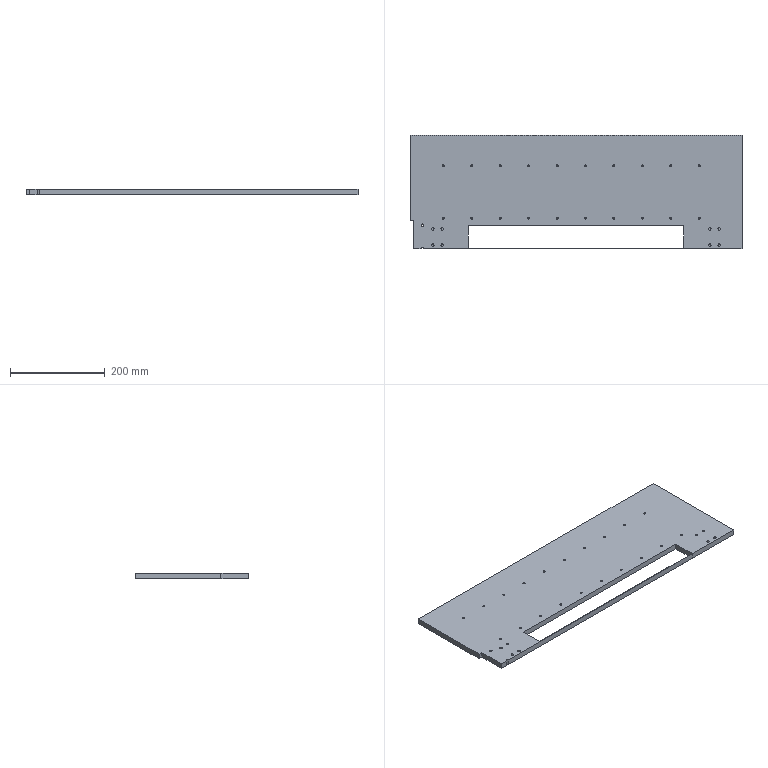Part | SolidWorks | features BaseBody 1 | 1 solid | 140 faces | box 700 x 240 x 12 mm | volume 1744066 mm3 | cylinder 99 | plane 41 | commonest cylinder face diameters 3.4 x40 4.3 x40 5.3 x19